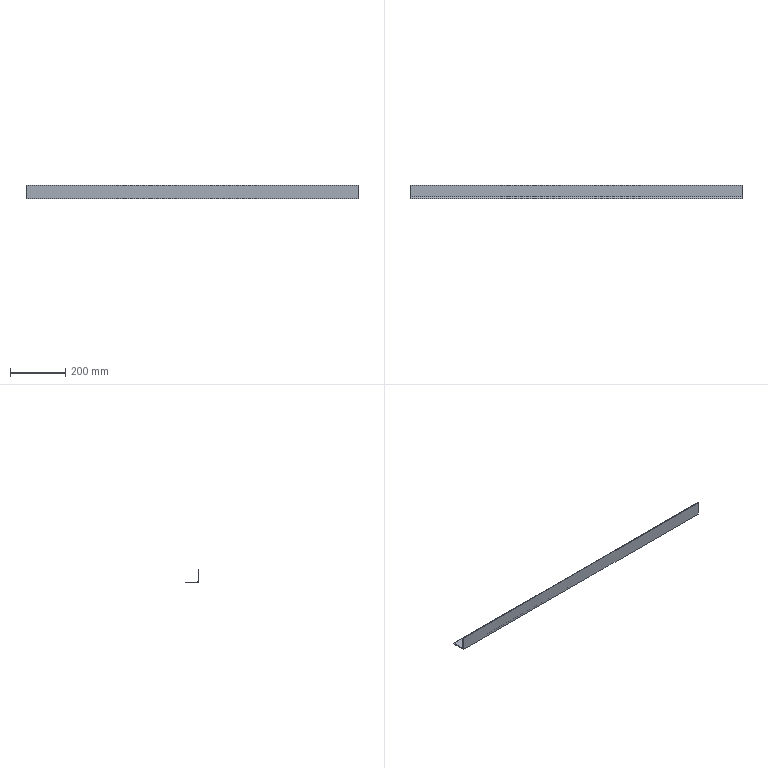Part | SolidWorks | features Extrusion 1 | 1 solid | 11 faces | box 1200 x 50 x 50 mm | volume 356475 mm3 | plane 8 | cylinder 3 | commonest cylinder face diameters 2 x2 11 x1
STEP:
#1=CARTESIAN_POINT('',(0.,2.,50.));
#2=VERTEX_POINT('',#1);
#3=CARTESIAN_POINT('',(0.,0.,50.));
#4=VERTEX_POINT('',#3);
#5=CARTESIAN_POINT('',(0.,0.,50.));
#6=DIRECTION('',(0.,-1.,0.));
#7=VECTOR('',#6,1000.);
#8=LINE('',#5,#7);
#9=EDGE_CURVE('',#2,#4,#8,.T.);
#10=ORIENTED_EDGE('',*,*,#9,.T.);
#11=CARTESIAN_POINT('',(1200.,0.,50.));
#12=VERTEX_POINT('',#11);
#13=CARTESIAN_POINT('',(1200.,0.,50.));
#14=DIRECTION('',(-1.,0.,0.));
#15=VECTOR('',#14,1000.);
#16=LINE('',#13,#15);
#17=EDGE_CURVE('',#12,#4,#16,.T.);
#18=ORIENTED_EDGE('',*,*,#17,.F.);
#19=CARTESIAN_POINT('',(1200.,2.,50.));
#20=VERTEX_POINT('',#19);
#21=CARTESIAN_POINT('',(1200.,0.,50.));
#22=DIRECTION('',(0.,-1.,0.));
#23=VECTOR('',#22,1000.);
#24=LINE('',#21,#23);
#25=EDGE_CURVE('',#20,#12,#24,.T.);
#26=ORIENTED_EDGE('',*,*,#25,.F.);
#27=CARTESIAN_POINT('',(1200.,2.,50.));
#28=DIRECTION('',(-1.,0.,0.));
#29=VECTOR('',#28,1000.);
#30=LINE('',#27,#29);
#31=EDGE_CURVE('',#20,#2,#30,.T.);
#32=ORIENTED_EDGE('',*,*,#31,.T.);
#33=EDGE_LOOP('',(#10,#18,#26,#32));
#34=FACE_OUTER_BOUND('',#33,.T.);
#35=CARTESIAN_POINT('',(1200.,0.,50.));
#36=DIRECTION('',(0.,0.,-1.));
#37=DIRECTION('',(-1.,0.,0.));
#38=AXIS2_PLACEMENT_3D('',#35,#36,#37);
#39=PLANE('',#38);
#40=ADVANCED_FACE('',(#34),#39,.F.);
#41=CARTESIAN_POINT('',(0.,0.,0.));
#42=VERTEX_POINT('',#41);
#43=CARTESIAN_POINT('',(0.,0.,50.));
#44=DIRECTION('',(0.,0.,-1.));
#45=VECTOR('',#44,1000.);
#46=LINE('',#43,#45);
#47=EDGE_CURVE('',#4,#42,#46,.T.);
#48=ORIENTED_EDGE('',*,*,#47,.T.);
#49=CARTESIAN_POINT('',(1200.,0.,0.));
#50=VERTEX_POINT('',#49);
#51=CARTESIAN_POINT('',(1200.,0.,0.));
#52=DIRECTION('',(-1.,0.,0.));
#53=VECTOR('',#52,1000.);
#54=LINE('',#51,#53);
#55=EDGE_CURVE('',#50,#42,#54,.T.);
#56=ORIENTED_EDGE('',*,*,#55,.F.);
#57=CARTESIAN_POINT('',(1200.,0.,50.));
#58=DIRECTION('',(0.,0.,-1.));
#59=VECTOR('',#58,1000.);
#60=LINE('',#57,#59);
#61=EDGE_CURVE('',#12,#50,#60,.T.);
#62=ORIENTED_EDGE('',*,*,#61,.F.);
#63=ORIENTED_EDGE('',*,*,#17,.T.);
#64=EDGE_LOOP('',(#48,#56,#62,#63));
#65=FACE_OUTER_BOUND('',#64,.T.);
#66=CARTESIAN_POINT('',(1200.,0.,50.));
#67=DIRECTION('',(0.,1.,0.));
#68=DIRECTION('',(0.,0.,1.));
#69=AXIS2_PLACEMENT_3D('',#66,#67,#68);
#70=PLANE('',#69);
#71=ADVANCED_FACE('',(#65),#70,.F.);
#72=CARTESIAN_POINT('',(0.,50.,0.));
#73=VERTEX_POINT('',#72);
#74=CARTESIAN_POINT('',(0.,0.,0.));
#75=DIRECTION('',(0.,1.,0.));
#76=VECTOR('',#75,1000.);
#77=LINE('',#74,#76);
#78=EDGE_CURVE('',#42,#73,#77,.T.);
#79=ORIENTED_EDGE('',*,*,#78,.T.);
#80=CARTESIAN_POINT('',(1200.,50.,0.));
#81=VERTEX_POINT('',#80);
#82=CARTESIAN_POINT('',(1200.,50.,0.));
#83=DIRECTION('',(-1.,0.,0.));
#84=VECTOR('',#83,1000.);
#85=LINE('',#82,#84);
#86=EDGE_CURVE('',#81,#73,#85,.T.);
#87=ORIENTED_EDGE('',*,*,#86,.F.);
#88=CARTESIAN_POINT('',(1200.,0.,0.));
#89=DIRECTION('',(0.,1.,0.));
#90=VECTOR('',#89,1000.);
#91=LINE('',#88,#90);
#92=EDGE_CURVE('',#50,#81,#91,.T.);
#93=ORIENTED_EDGE('',*,*,#92,.F.);
#94=ORIENTED_EDGE('',*,*,#55,.T.);
#95=EDGE_LOOP('',(#79,#87,#93,#94));
#96=FACE_OUTER_BOUND('',#95,.T.);
#97=CARTESIAN_POINT('',(1200.,0.,0.));
#98=DIRECTION('',(0.,0.,1.));
#99=DIRECTION('',(1.,0.,0.));
#100=AXIS2_PLACEMENT_3D('',#97,#98,#99);
#101=PLANE('',#100);
#102=ADVANCED_FACE('',(#96),#101,.F.);
#103=CARTESIAN_POINT('',(0.,50.,2.));
#104=VERTEX_POINT('',#103);
#105=CARTESIAN_POINT('',(0.,50.,0.));
#106=DIRECTION('',(0.,0.,1.));
#107=VECTOR('',#106,1000.);
#108=LINE('',#105,#107);
#109=EDGE_CURVE('',#73,#104,#108,.T.);
#110=ORIENTED_EDGE('',*,*,#109,.T.);
#111=CARTESIAN_POINT('',(1200.,50.,2.));
#112=VERTEX_POINT('',#111);
#113=CARTESIAN_POINT('',(1200.,50.,2.));
#114=DIRECTION('',(-1.,0.,0.));
#115=VECTOR('',#114,1000.);
#116=LINE('',#113,#115);
#117=EDGE_CURVE('',#112,#104,#116,.T.);
#118=ORIENTED_EDGE('',*,*,#117,.F.);
#119=CARTESIAN_POINT('',(1200.,50.,0.));
#120=DIRECTION('',(0.,0.,1.));
#121=VECTOR('',#120,1000.);
#122=LINE('',#119,#121);
#123=EDGE_CURVE('',#81,#112,#122,.T.);
#124=ORIENTED_EDGE('',*,*,#123,.F.);
#125=ORIENTED_EDGE('',*,*,#86,.T.);
#126=EDGE_LOOP('',(#110,#118,#124,#125));
#127=FACE_OUTER_BOUND('',#126,.T.);
#128=CARTESIAN_POINT('',(1200.,50.,0.));
#129=DIRECTION('',(0.,-1.,0.));
#130=DIRECTION('',(0.,0.,-1.));
#131=AXIS2_PLACEMENT_3D('',#128,#129,#130);
#132=PLANE('',#131);
#133=ADVANCED_FACE('',(#127),#132,.F.);
#134=CARTESIAN_POINT('',(0.,49.,3.));
#135=VERTEX_POINT('',#134);
#136=CARTESIAN_POINT('',(0.,49.,2.));
#137=DIRECTION('',(1.,0.,0.));
#138=DIRECTION('',(0.,0.,-1.));
#139=AXIS2_PLACEMENT_3D('',#136,#137,#138);
#140=CIRCLE('',#139,1.);
#141=EDGE_CURVE('',#104,#135,#140,.T.);
#142=ORIENTED_EDGE('',*,*,#141,.T.);
#143=CARTESIAN_POINT('',(1200.,49.,3.));
#144=VERTEX_POINT('',#143);
#145=CARTESIAN_POINT('',(1200.,49.,3.));
#146=DIRECTION('',(-1.,0.,0.));
#147=VECTOR('',#146,1000.);
#148=LINE('',#145,#147);
#149=EDGE_CURVE('',#144,#135,#148,.T.);
#150=ORIENTED_EDGE('',*,*,#149,.F.);
#151=CARTESIAN_POINT('',(1200.,49.,2.));
#152=DIRECTION('',(1.,0.,0.));
#153=DIRECTION('',(0.,0.,-1.));
#154=AXIS2_PLACEMENT_3D('',#151,#152,#153);
#155=CIRCLE('',#154,1.);
#156=EDGE_CURVE('',#112,#144,#155,.T.);
#157=ORIENTED_EDGE('',*,*,#156,.F.);
#158=ORIENTED_EDGE('',*,*,#117,.T.);
#159=EDGE_LOOP('',(#142,#150,#157,#158));
#160=FACE_OUTER_BOUND('',#159,.T.);
#161=CARTESIAN_POINT('',(1200.,49.,2.));
#162=DIRECTION('',(-1.,0.,0.));
#163=DIRECTION('',(0.,0.,1.));
#164=AXIS2_PLACEMENT_3D('',#161,#162,#163);
#165=CYLINDRICAL_SURFACE('',#164,1.);
#166=ADVANCED_FACE('',(#160),#165,.T.);
#167=CARTESIAN_POINT('',(0.,8.5,3.));
#168=VERTEX_POINT('',#167);
#169=CARTESIAN_POINT('',(0.,8.5,3.));
#170=DIRECTION('',(0.,-1.,0.));
#171=VECTOR('',#170,1000.);
#172=LINE('',#169,#171);
#173=EDGE_CURVE('',#135,#168,#172,.T.);
#174=ORIENTED_EDGE('',*,*,#173,.T.);
#175=CARTESIAN_POINT('',(1200.,8.5,3.));
#176=VERTEX_POINT('',#175);
#177=CARTESIAN_POINT('',(1200.,8.5,3.));
#178=DIRECTION('',(-1.,0.,0.));
#179=VECTOR('',#178,1000.);
#180=LINE('',#177,#179);
#181=EDGE_CURVE('',#176,#168,#180,.T.);
#182=ORIENTED_EDGE('',*,*,#181,.F.);
#183=CARTESIAN_POINT('',(1200.,8.5,3.));
#184=DIRECTION('',(0.,-1.,0.));
#185=VECTOR('',#184,1000.);
#186=LINE('',#183,#185);
#187=EDGE_CURVE('',#144,#176,#186,.T.);
#188=ORIENTED_EDGE('',*,*,#187,.F.);
#189=ORIENTED_EDGE('',*,*,#149,.T.);
#190=EDGE_LOOP('',(#174,#182,#188,#189));
#191=FACE_OUTER_BOUND('',#190,.T.);
#192=CARTESIAN_POINT('',(1200.,8.5,3.));
#193=DIRECTION('',(0.,0.,-1.));
#194=DIRECTION('',(0.,1.,0.));
#195=AXIS2_PLACEMENT_3D('',#192,#193,#194);
#196=PLANE('',#195);
#197=ADVANCED_FACE('',(#191),#196,.F.);
#198=CARTESIAN_POINT('',(0.,3.,8.5));
#199=VERTEX_POINT('',#198);
#200=CARTESIAN_POINT('',(0.,8.5,8.5));
#201=DIRECTION('',(-1.,0.,0.));
#202=DIRECTION('',(0.,0.,-1.));
#203=AXIS2_PLACEMENT_3D('',#200,#201,#202);
#204=CIRCLE('',#203,5.5);
#205=EDGE_CURVE('',#168,#199,#204,.T.);
#206=ORIENTED_EDGE('',*,*,#205,.T.);
#207=CARTESIAN_POINT('',(1200.,3.,8.5));
#208=VERTEX_POINT('',#207);
#209=CARTESIAN_POINT('',(1200.,3.,8.5));
#210=DIRECTION('',(-1.,0.,0.));
#211=VECTOR('',#210,1000.);
#212=LINE('',#209,#211);
#213=EDGE_CURVE('',#208,#199,#212,.T.);
#214=ORIENTED_EDGE('',*,*,#213,.F.);
#215=CARTESIAN_POINT('',(1200.,8.5,8.5));
#216=DIRECTION('',(-1.,0.,0.));
#217=DIRECTION('',(0.,0.,-1.));
#218=AXIS2_PLACEMENT_3D('',#215,#216,#217);
#219=CIRCLE('',#218,5.5);
#220=EDGE_CURVE('',#176,#208,#219,.T.);
#221=ORIENTED_EDGE('',*,*,#220,.F.);
#222=ORIENTED_EDGE('',*,*,#181,.T.);
#223=EDGE_LOOP('',(#206,#214,#221,#222));
#224=FACE_OUTER_BOUND('',#223,.T.);
#225=CARTESIAN_POINT('',(1200.,8.5,8.5));
#226=DIRECTION('',(-1.,0.,0.));
#227=DIRECTION('',(0.,0.,1.));
#228=AXIS2_PLACEMENT_3D('',#225,#226,#227);
#229=CYLINDRICAL_SURFACE('',#228,5.5);
#230=ADVANCED_FACE('',(#224),#229,.F.);
#231=CARTESIAN_POINT('',(0.,3.,49.));
#232=VERTEX_POINT('',#231);
#233=CARTESIAN_POINT('',(0.,3.,49.));
#234=DIRECTION('',(0.,0.,1.));
#235=VECTOR('',#234,1000.);
#236=LINE('',#233,#235);
#237=EDGE_CURVE('',#199,#232,#236,.T.);
#238=ORIENTED_EDGE('',*,*,#237,.T.);
#239=CARTESIAN_POINT('',(1200.,3.,49.));
#240=VERTEX_POINT('',#239);
#241=CARTESIAN_POINT('',(1200.,3.,49.));
#242=DIRECTION('',(-1.,0.,0.));
#243=VECTOR('',#242,1000.);
#244=LINE('',#241,#243);
#245=EDGE_CURVE('',#240,#232,#244,.T.);
#246=ORIENTED_EDGE('',*,*,#245,.F.);
#247=CARTESIAN_POINT('',(1200.,3.,49.));
#248=DIRECTION('',(0.,0.,1.));
#249=VECTOR('',#248,1000.);
#250=LINE('',#247,#249);
#251=EDGE_CURVE('',#208,#240,#250,.T.);
#252=ORIENTED_EDGE('',*,*,#251,.F.);
#253=ORIENTED_EDGE('',*,*,#213,.T.);
#254=EDGE_LOOP('',(#238,#246,#252,#253));
#255=FACE_OUTER_BOUND('',#254,.T.);
#256=CARTESIAN_POINT('',(1200.,3.,49.));
#257=DIRECTION('',(0.,-1.,0.));
#258=DIRECTION('',(0.,0.,-1.));
#259=AXIS2_PLACEMENT_3D('',#256,#257,#258);
#260=PLANE('',#259);
#261=ADVANCED_FACE('',(#255),#260,.F.);
#262=CARTESIAN_POINT('',(0.,2.,49.));
#263=DIRECTION('',(1.,0.,0.));
#264=DIRECTION('',(0.,0.,1.));
#265=AXIS2_PLACEMENT_3D('',#262,#263,#264);
#266=CIRCLE('',#265,1.);
#267=EDGE_CURVE('',#232,#2,#266,.T.);
#268=ORIENTED_EDGE('',*,*,#267,.T.);
#269=ORIENTED_EDGE('',*,*,#31,.F.);
#270=CARTESIAN_POINT('',(1200.,2.,49.));
#271=DIRECTION('',(1.,0.,0.));
#272=DIRECTION('',(0.,0.,1.));
#273=AXIS2_PLACEMENT_3D('',#270,#271,#272);
#274=CIRCLE('',#273,1.);
#275=EDGE_CURVE('',#240,#20,#274,.T.);
#276=ORIENTED_EDGE('',*,*,#275,.F.);
#277=ORIENTED_EDGE('',*,*,#245,.T.);
#278=EDGE_LOOP('',(#268,#269,#276,#277));
#279=FACE_OUTER_BOUND('',#278,.T.);
#280=CARTESIAN_POINT('',(1200.,2.,49.));
#281=DIRECTION('',(-1.,0.,0.));
#282=DIRECTION('',(0.,0.,1.));
#283=AXIS2_PLACEMENT_3D('',#280,#281,#282);
#284=CYLINDRICAL_SURFACE('',#283,1.);
#285=ADVANCED_FACE('',(#279),#284,.T.);
#286=ORIENTED_EDGE('',*,*,#25,.T.);
#287=ORIENTED_EDGE('',*,*,#61,.T.);
#288=ORIENTED_EDGE('',*,*,#92,.T.);
#289=ORIENTED_EDGE('',*,*,#123,.T.);
#290=ORIENTED_EDGE('',*,*,#156,.T.);
#291=ORIENTED_EDGE('',*,*,#187,.T.);
#292=ORIENTED_EDGE('',*,*,#220,.T.);
#293=ORIENTED_EDGE('',*,*,#251,.T.);
#294=ORIENTED_EDGE('',*,*,#275,.T.);
#295=EDGE_LOOP('',(#286,#287,#288,#289,#290,#291,#292,#293,#294));
#296=FACE_OUTER_BOUND('',#295,.T.);
#297=CARTESIAN_POINT('',(1200.,2.,49.));
#298=DIRECTION('',(-1.,0.,0.));
#299=DIRECTION('',(0.,0.,1.));
#300=AXIS2_PLACEMENT_3D('',#297,#298,#299);
#301=PLANE('',#300);
#302=ADVANCED_FACE('',(#296),#301,.F.);
#303=ORIENTED_EDGE('',*,*,#9,.F.);
#304=ORIENTED_EDGE('',*,*,#267,.F.);
#305=ORIENTED_EDGE('',*,*,#237,.F.);
#306=ORIENTED_EDGE('',*,*,#205,.F.);
#307=ORIENTED_EDGE('',*,*,#173,.F.);
#308=ORIENTED_EDGE('',*,*,#141,.F.);
#309=ORIENTED_EDGE('',*,*,#109,.F.);
#310=ORIENTED_EDGE('',*,*,#78,.F.);
#311=ORIENTED_EDGE('',*,*,#47,.F.);
#312=EDGE_LOOP('',(#303,#304,#305,#306,#307,#308,#309,#310,#311));
#313=FACE_OUTER_BOUND('',#312,.T.);
#314=CARTESIAN_POINT('',(0.,2.,49.));
#315=DIRECTION('',(-1.,0.,0.));
#316=DIRECTION('',(0.,0.,1.));
#317=AXIS2_PLACEMENT_3D('',#314,#315,#316);
#318=PLANE('',#317);
#319=ADVANCED_FACE('',(#313),#318,.T.);
#320=CLOSED_SHELL('',(#40,#71,#102,#133,#166,#197,#230,#261,#285,#302,#319));
#321=MANIFOLD_SOLID_BREP('',#320);
#322=CARTESIAN_POINT('',(0.,0.,0.));
#323=DIRECTION('',(0.,0.,1.));
#324=DIRECTION('',(1.,0.,0.));
#325=AXIS2_PLACEMENT_3D('',#322,#323,#324);
#326=(LENGTH_UNIT()NAMED_UNIT(*)SI_UNIT(.MILLI.,.METRE.));
#327=UNCERTAINTY_MEASURE_WITH_UNIT(LENGTH_MEASURE(0.00001),#326,'','');
#328=(NAMED_UNIT(*)PLANE_ANGLE_UNIT()SI_UNIT($,.RADIAN.));
#329=(NAMED_UNIT(*)SI_UNIT($,.STERADIAN.)SOLID_ANGLE_UNIT());
#330=(GEOMETRIC_REPRESENTATION_CONTEXT(3)GLOBAL_UNCERTAINTY_ASSIGNED_CONTEXT((#327))GLOBAL_UNIT_ASSIGNED_CONTEXT((#326,#328,#329))REPRESENTATION_CONTEXT('',''));
#331=ADVANCED_BREP_SHAPE_REPRESENTATION('',(#321,#325),#330);